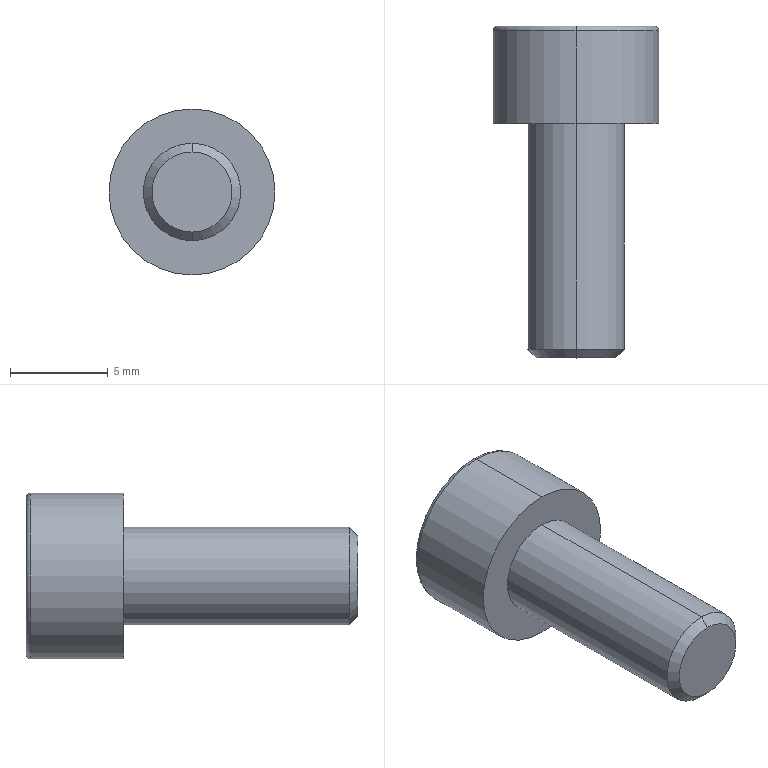Part | STEP file | hex socket M5x12 | 1 solid | 20 faces | box 8.5 x 17 x 8.5 mm | volume 481.648 mm3 | plane 10 | cone 4 | cylinder 4 | torus 2 | commonest cylinder face diameters 5 x2 8.5 x2